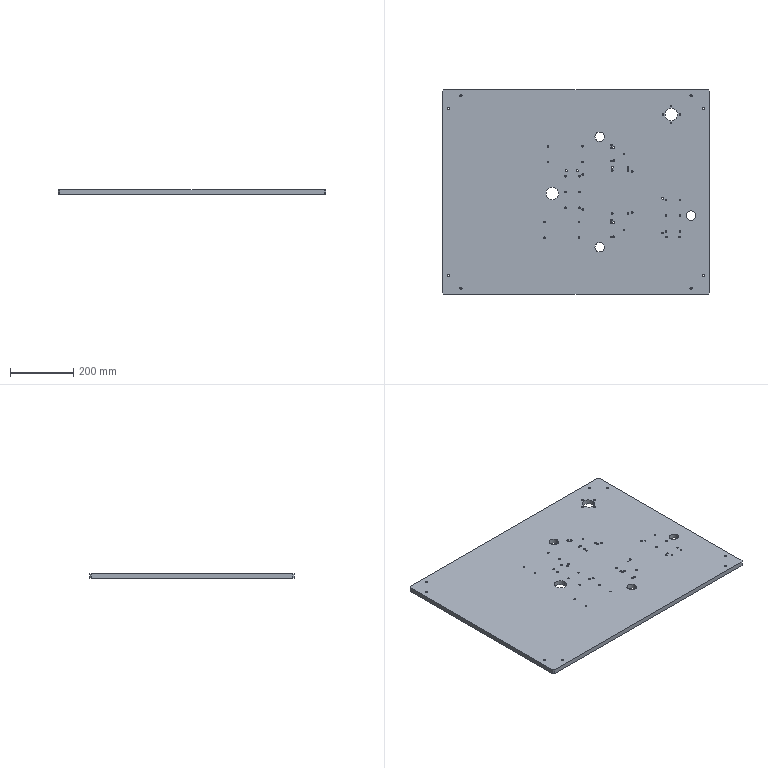Part | STEP file | Base plate | 1 solid | 164 faces | box 850 x 650 x 15 mm | volume 8193242 mm3 | cylinder 146 | plane 18 | commonest cylinder face diameters 5 x48 6 x36 4.2 x20 6.6 x16 11 x16 30 x6